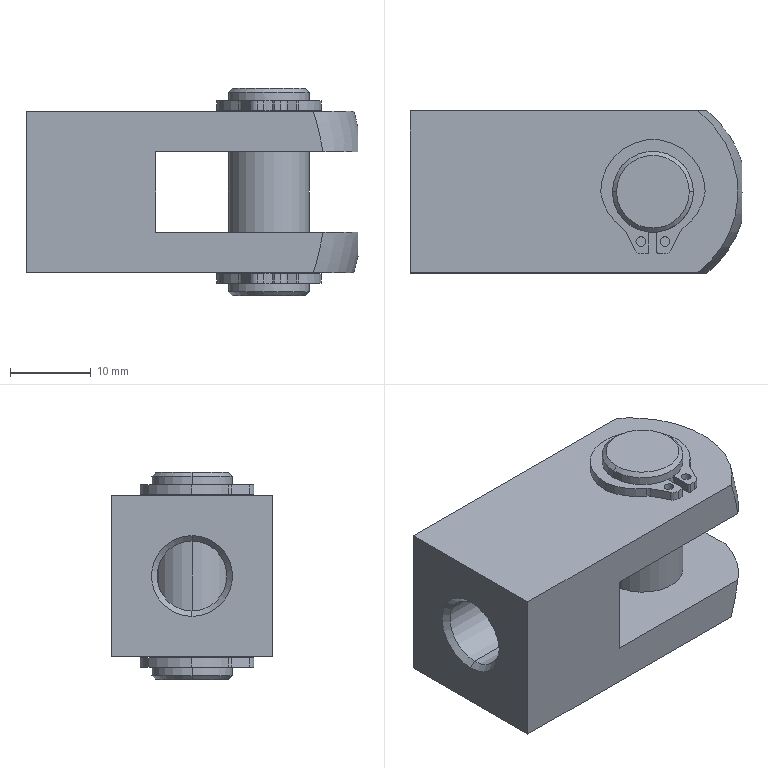Part | SolidWorks | features BaseBody 1 | 1 solid | 87 faces | box 41 x 20 x 25.6 mm | volume 11481 mm3 | cylinder 46 | plane 33 | cone 6 | torus 2 | commonest cylinder face diameters 10 x10 1.2 x8 2 x8 0.4 x4 1 x4 13.013 x4